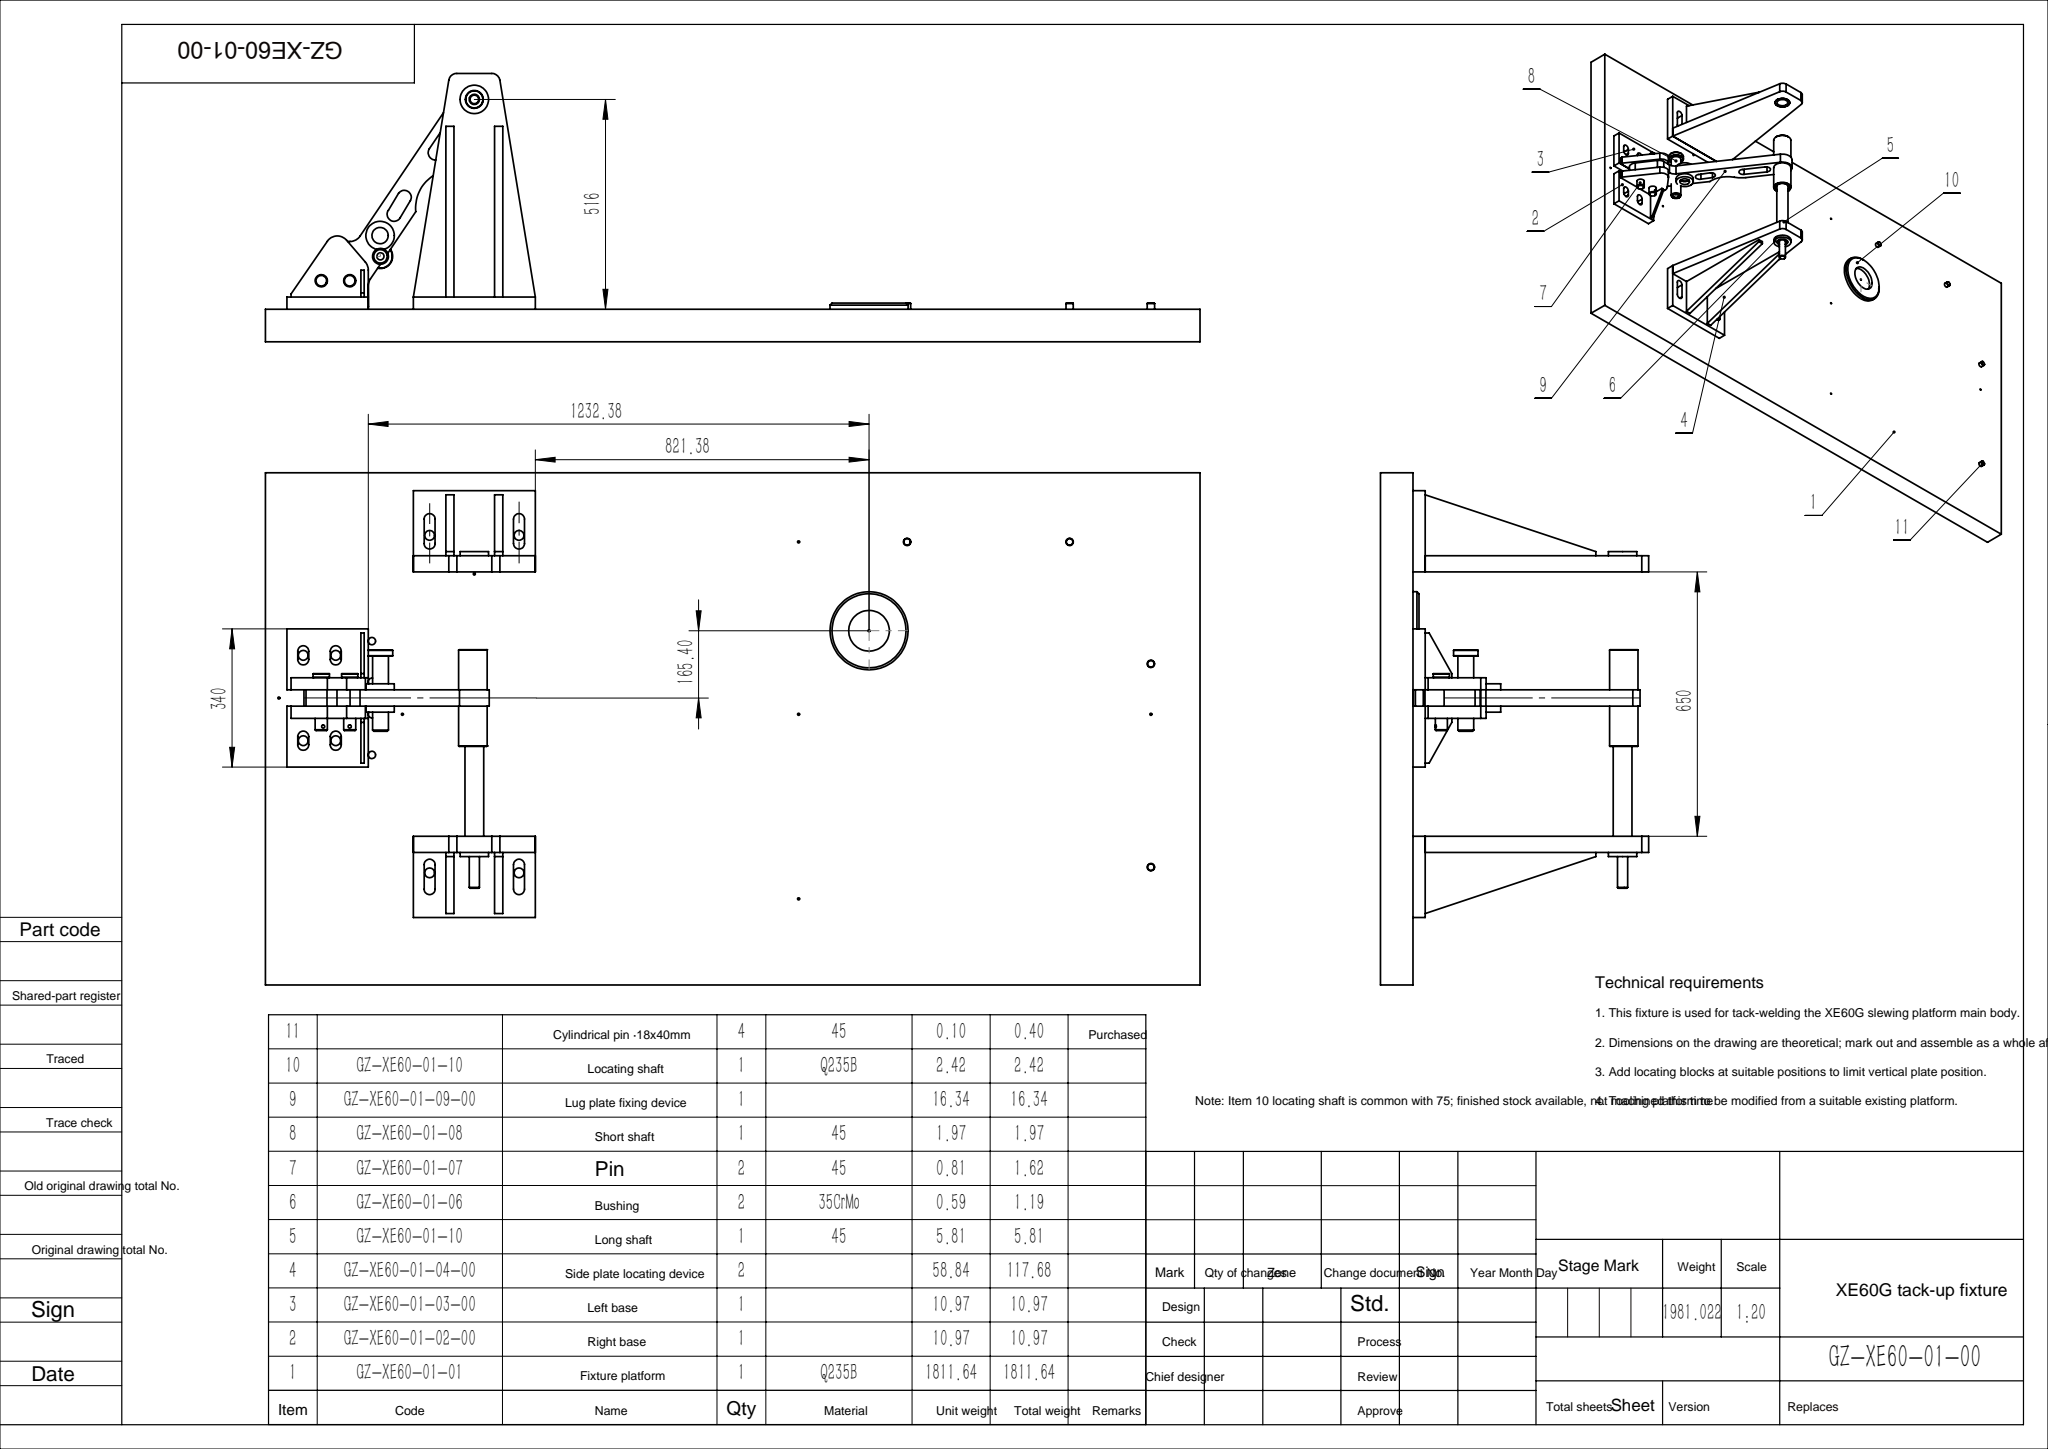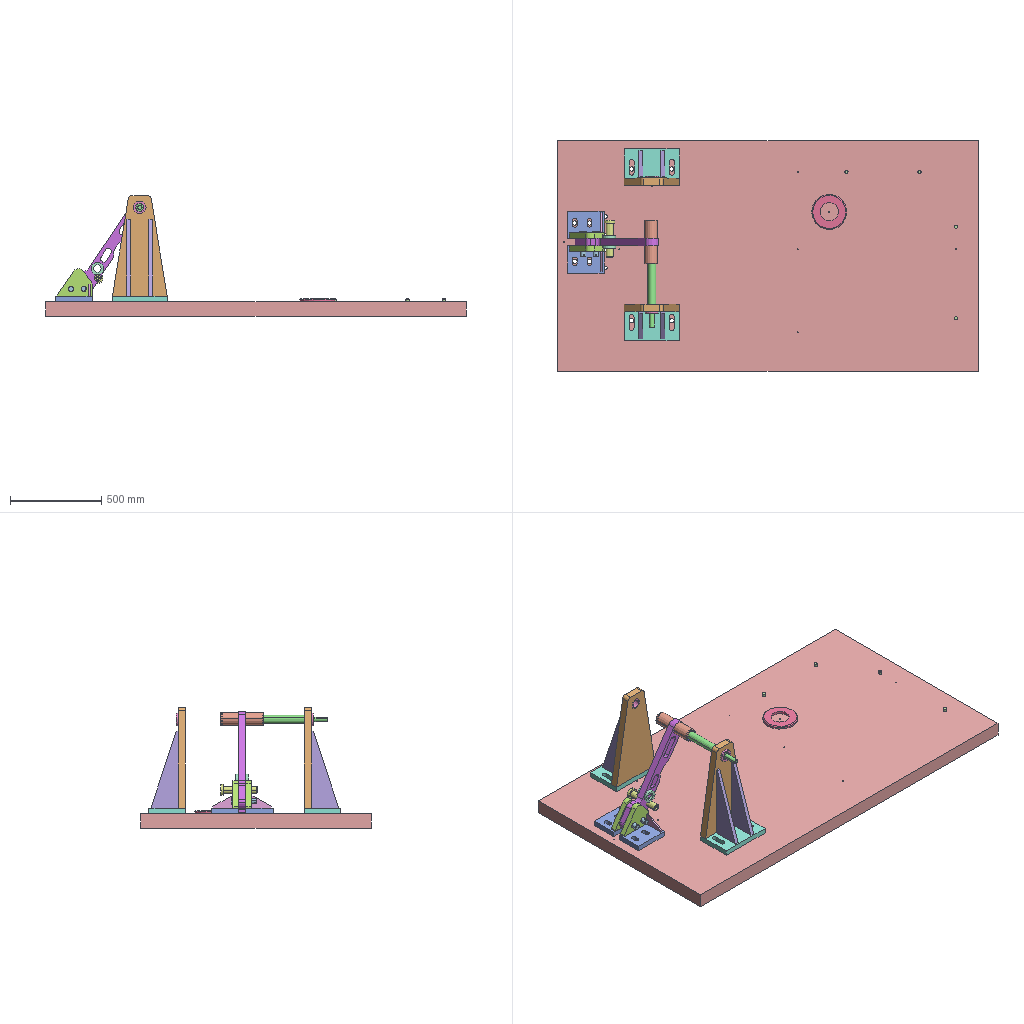Assembly | SolidWorks | 22 different items | 38 placed | box 2300 x 1260 x 660 mm
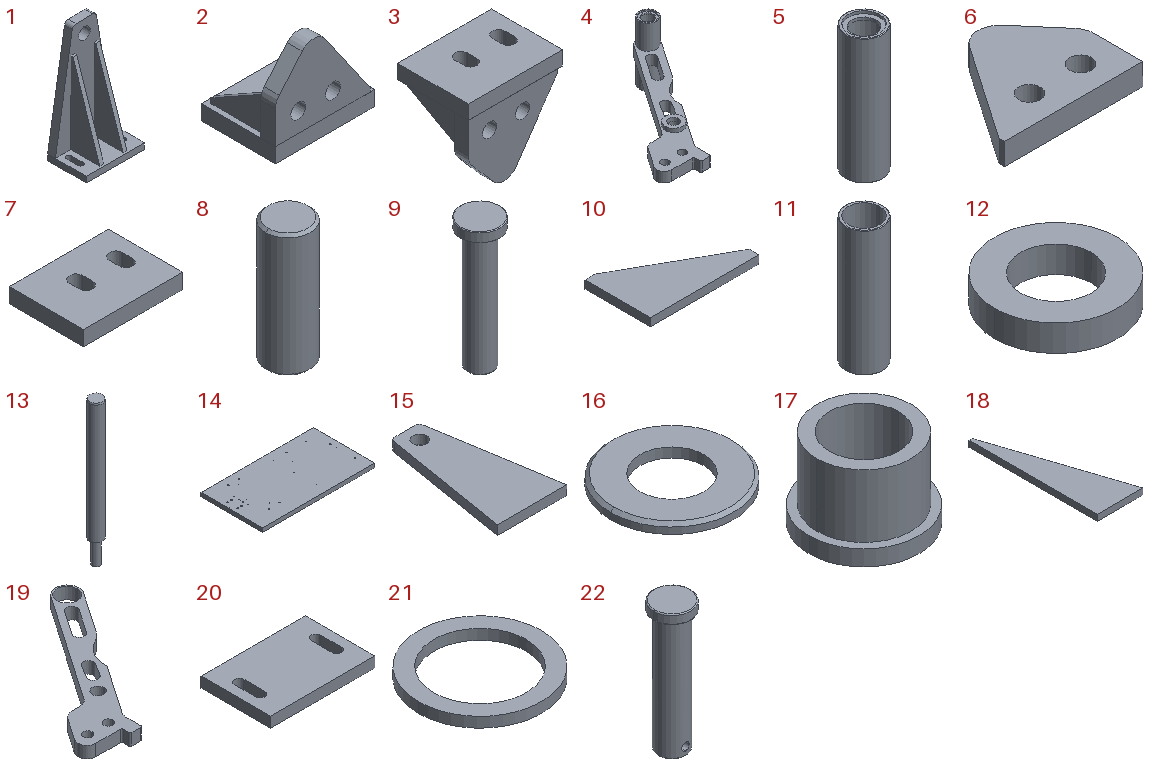Parts list (item | name | quantity | parent item | size | volume | features):
1 | (subassembly) | x2 | - | 300 x 200 x 580 mm | 7514698 mm3 | -
2 | (subassembly) | x1 | - | 200 x 150 x 180.029 mm | 1401678 mm3 | -
3 | (subassembly) | x1 | - | 200 x 150 x 180.029 mm | 1401678 mm3 | -
4 | (subassembly) | x1 | - | 459.333 x 555.5 x 238 mm | 2086739 mm3 | -
5 | (subassembly) | x1 | in 4 | 70 x 70 x 238 mm | 255154 mm3 | -
6 | - | x2 | in 2, 3 | 190 x 150.029 x 30 mm | 532752 mm3 | features Extrusion 1
7 | - | x2 | in 2, 3 | 200 x 150 x 30 mm | 833247 mm3 | features Extrusion 1
8 | - | x4 | - | 18 x 18 x 50 mm | 12669 mm3 | features Chamfer 1, Extrusion 1
9 | - | x1 | - | 60 x 60 x 200 mm | 249652 mm3 | features Chamfer 2, 3DProfileFeature 1, Extrusion 1, HoleWzd 1, ICE 1
10 | - | x2 | in 2, 3 | 110 x 66 x 8 mm | 35680 mm3 | features Extrusion 1
11 | - | x1 | in 5 | 70 x 70 x 238 mm | 242784 mm3 | features Chamfer 1, Extrusion 1
12 | - | x2 | in 4 | 70 x 70 x 15 mm | 38877 mm3 | features Extrusion 1
13 | - | x1 | - | 46 x 46 x 500 mm | 736365 mm3 | features Chamfer 2, Extrusion 1, ICE 1
14 | - | x1 | - | 2300 x 1260 x 80 mm | 231371903 mm3 | features Extrusion 1
15 | - | x2 | in 1 | 300 x 550 x 40 mm | 4502251 mm3 | features Extrusion 1
16 | - | x1 | - | 192 x 192 x 15 mm | 309075 mm3 | features Chamfer 1, Extrusion 1
17 | - | x2 | - | 70 x 70 x 50 mm | 75555 mm3 | features Extrusion 1, ICE 1
18 | - | x4 | in 1 | 150 x 420 x 20 mm | 672000 mm3 | features Extrusion 1
19 | - | x1 | in 4 | 459.333 x 555.5 x 40 mm | 1753830 mm3 | features Extrusion 1
20 | - | x2 | in 1 | 300 x 200 x 30 mm | 1668447 mm3 | features Extrusion 1
21 | - | x2 | in 5 | 60 x 60 x 5 mm | 6185 mm3 | features Extrusion 1
22 | - | x2 | - | 40 x 40 x 140 mm | 102751 mm3 | features Fillet 2, ICE 2, Chamfer 1, Extrusion 1
Mates (type | each side: item.copy, entity, surface, feature):
In the top assembly
Tangent | 14.1 face cylinder Boss-Extrude1 | assembly face | 3 times
Coincident | 14.1 face plane Boss-Extrude1 | assembly face
Coincident | 14.1 face plane Boss-Extrude1 | 7.1 face plane Boss-Extrude1
Coincident | 14.1 face plane Boss-Extrude1 | 7.2 face plane Boss-Extrude1
Concentric | 6.1 face cylinder Boss-Extrude1 | 6.2 face cylinder Boss-Extrude1
DistanceDim | 7.2 face plane Boss-Extrude1 | assembly face
Coincident | 14.1 face plane Boss-Extrude1 | 20.1 face plane Boss-Extrude1
Parallel | assembly face | 15.1 face cylinder Boss-Extrude1
Coincident | 14.1 face plane Boss-Extrude1 | 20.2 face plane Boss-Extrude1
Concentric | assembly face | 15.1 face cylinder Boss-Extrude1
Concentric | assembly face | 15.2 face cylinder Boss-Extrude1
DistanceDim | assembly face | 15.2 face plane Boss-Extrude1
DistanceDim | 15.1 face plane Boss-Extrude1 | assembly face
Concentric | assembly face | 13.1 face cylinder Boss-Extrude1
Coincident | 14.1 face plane Boss-Extrude1 | 16.1 face plane Boss-Extrude1
Concentric | assembly face | 16.1 face cylinder Boss-Extrude1
Concentric | 6.1 face cylinder Boss-Extrude1 | 22.1 face cylinder Boss-Extrude1
Concentric | 6.1 face cylinder Boss-Extrude1 | 22.2 face cylinder Boss-Extrude1
Coincident | 6.2 face plane Boss-Extrude1 | 22.2 face plane Boss-Extrude2
Concentric | assembly face | 9.1 face cylinder Boss-Extrude1
Coincident | 6.2 face plane Boss-Extrude1 | 22.1 face plane Boss-Extrude2
Concentric | assembly face | assembly face
DistanceDim | 12.1 face plane Boss-Extrude1 | assembly face
Coincident | 6.1 face plane Boss-Extrude1 | 19.1 face plane Boss-Extrude1
Coincident | 6.2 face plane Boss-Extrude1 | 19.1 face plane Boss-Extrude1
Concentric | 22.1 face cylinder Boss-Extrude1 | 19.1 face cylinder Boss-Extrude1
Concentric | 14.1 face cylinder Boss-Extrude1 | 8.1 face cylinder Boss-Extrude1
Concentric | 14.1 face cylinder Boss-Extrude1 | 8.2 face cylinder Boss-Extrude1
Concentric | 14.1 face cylinder Boss-Extrude1 | 8.3 face cylinder Boss-Extrude1
Concentric | 14.1 face cylinder Boss-Extrude1 | 8.4 face cylinder Boss-Extrude1
DistanceDim | 8.4 face plane Boss-Extrude1 | 14.1 face plane Boss-Extrude1
DistanceDim | 8.3 face plane Boss-Extrude1 | 14.1 face plane Boss-Extrude1
DistanceDim | 8.2 face plane Boss-Extrude1 | 14.1 face plane Boss-Extrude1
DistanceDim | 8.1 face plane Boss-Extrude1 | 14.1 face plane Boss-Extrude1
Concentric | 15.2 face cylinder Boss-Extrude1 | 17.1 face cylinder Boss-Extrude1
Coincident | 15.2 face plane Boss-Extrude1 | 17.1 face plane Boss-Extrude2
Concentric | 15.1 face cylinder Boss-Extrude1 | 17.2 face cylinder Boss-Extrude1
Coincident | 15.1 face plane Boss-Extrude1 | 17.2 face plane Boss-Extrude2
In subassembly 4
Concentric | 19.2 face cylinder Boss-Extrude1 | 4.1 face
Coincident | 19.2 face plane Boss-Extrude1 | 4.1 face
Coincident | 19.2 face plane Boss-Extrude1 | 12.2 face plane Boss-Extrude1
Concentric | 19.2 face cylinder Boss-Extrude1 | 12.2 face cylinder Boss-Extrude1
Coincident | 19.2 face plane Boss-Extrude1 | 12.3 face plane Boss-Extrude1
Concentric | 19.2 face cylinder Boss-Extrude1 | 12.3 face cylinder Boss-Extrude1
Concentric | 19.2 face cylinder Boss-Extrude1 | 11.1 face cylinder Boss-Extrude1
DistanceDim | 11.1 face plane Boss-Extrude1 | 12.3 face plane Boss-Extrude1
In subassembly 5
DistanceDim | 11.2 face plane Boss-Extrude1 | 21.1 face plane Boss-Extrude1
Concentric | 11.2 face cylinder Boss-Extrude1 | 21.1 face cylinder Boss-Extrude1
Concentric | 11.2 face cylinder Boss-Extrude1 | 21.2 face cylinder Boss-Extrude1
DistanceDim | 11.2 face plane Boss-Extrude1 | 21.2 face plane Boss-Extrude1
In subassembly 1
Coincident | 20.3 face plane Boss-Extrude1 | 15.3 face plane Boss-Extrude1 | 2 times
Coincident | 20.3 edge | 15.3 edge
Coincident | 20.3 face plane Boss-Extrude1 | 18.1 face plane Boss-Extrude1
Coincident | 15.3 face plane Boss-Extrude1 | 18.1 face plane Boss-Extrude1
Coincident | 20.3 face plane Boss-Extrude1 | 18.2 face plane Boss-Extrude1
Coincident | 15.3 face plane Boss-Extrude1 | 18.2 face plane Boss-Extrude1
DistanceDim | 18.2 face plane Boss-Extrude1 | 20.3 face plane Boss-Extrude1
DistanceDim | 18.1 face plane Boss-Extrude1 | 20.3 face plane Boss-Extrude1
Coincident | 15.3 face plane Boss-Extrude1 | 1.1 face
Concentric | 15.3 face cylinder Boss-Extrude1 | 1.1 face
In subassembly 2
Coincident | 7.3 face plane Boss-Extrude1 | 6.3 face plane Boss-Extrude1 | 3 times
Coincident | 6.3 face plane Boss-Extrude1 | 10.1 face plane Boss-Extrude1
Coincident | 7.3 face plane Boss-Extrude1 | 10.1 face plane Boss-Extrude1
DistanceDim | 7.3 face plane Boss-Extrude1 | 10.1 face plane Boss-Extrude1
In subassembly 3
Coincident | 7.3 face plane Boss-Extrude1 | 6.3 face plane Boss-Extrude1 | 3 times
Coincident | 6.3 face plane Boss-Extrude1 | 10.1 face plane Boss-Extrude1
Coincident | 7.3 face plane Boss-Extrude1 | 10.1 face plane Boss-Extrude1
DistanceDim | 6.3 face plane Boss-Extrude1 | 10.1 face plane Boss-Extrude1